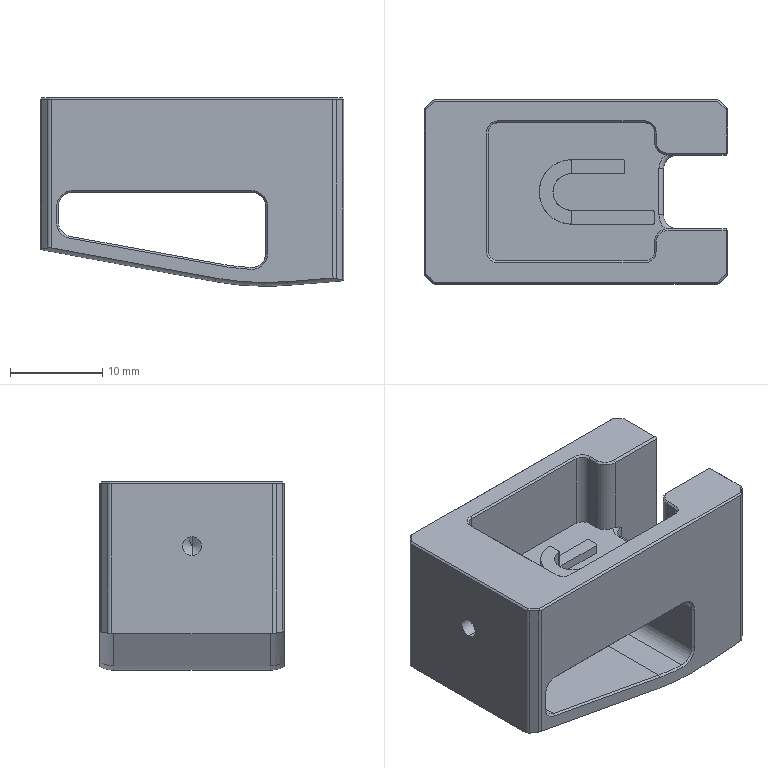NC program | NX | posted with a generic post | part box 33 x 20 x 20.478 mm
Lines 1298 to 2252 of 7616:
(FIXED_CONTOUR_COPY , TOOL : D2R0.5)
N2588 T24 M6
N2590 G54
N2592 G17 G0 G90 X-4.289 Y-10.746 B0. C0. S9500 M3
N2594 G43 Z30. H24
N2596 Z2.8
N2598 G94 G1 Z0.346 F1000.
N2600 X-4.343 Z0.091
N2602 X-4.461 Z-0.142
N2604 X-4.636 Z-0.336
N2606 X-4.854 Z-0.479
N2608 X-5.102 Z-0.56
N2610 X-5.363 Y-10.745 Z-0.574
N2612 X-5.715 Z-0.547 F2500.
N2614 X-6.315 Z-0.509
N2616 X-6.915 Y-10.744 Z-0.483
N2618 X-7.515 Z-0.47
N2620 X-8.115 Z-0.466
N2622 X-8.715 Y-10.743 Z-0.477
N2624 X-9.315 Z-0.496
N2626 X-9.915 Y-10.742 Z-0.532
N2628 X-10.515 Z-0.572
N2630 X-11.115 Z-0.62
N2632 X-11.715 Y-10.741 Z-0.668
N2634 X-12.315 Z-0.716
N2636 X-12.915 Y-10.74 Z-0.764
N2638 X-13.515 Z-0.812
N2640 X-14.115 Z-0.86
N2642 X-14.715 Y-10.739 Z-0.908
N2644 X-15.315 Z-0.956
N2646 X-15.495 Z-0.97
N2648 X-15.537 Y-10.719 Z-0.963
N2650 X-15.618 Y-10.705 Z-0.961
N2652 X-15.681 Y-10.646 Z-0.934
N2654 X-15.315 Z-0.905
N2656 X-14.715 Y-10.647 Z-0.857
N2658 X-14.115 Z-0.809
N2660 X-13.515 Z-0.762
N2662 X-12.915 Y-10.648 Z-0.714
N2664 X-12.315 Z-0.666
N2666 X-11.715 Y-10.649 Z-0.618
N2668 X-11.115 Z-0.57
N2670 X-10.515 Z-0.522
N2672 X-9.915 Y-10.65 Z-0.482
N2674 X-9.315 Z-0.446
N2676 X-8.715 Y-10.651 Z-0.428
N2678 X-8.115 Z-0.418
N2680 X-7.515 Z-0.42
N2682 X-6.915 Y-10.652 Z-0.435
N2684 X-6.315 Z-0.459
N2686 X-5.715 Y-10.653 Z-0.498
N2688 X-5.115 Z-0.547
N2690 X-4.515 Z-0.607
N2692 X-3.915 Y-10.654 Z-0.682
N2694 X-3.315 Z-0.765
N2696 X-2.715 Y-10.655 Z-0.865
N2698 X-2.115 Z-0.969
N2700 X-1.515 Z-1.08
N2702 X-0.915 Y-10.656 Z-1.19
N2704 X-0.315 Z-1.3
N2706 X0.285 Y-10.657 Z-1.411
N2708 X0.885 Z-1.521
N2710 X1.485 Z-1.631
N2712 X2.085 Y-10.658 Z-1.742
N2714 X2.685 Z-1.852
N2716 X3.285 Y-10.659 Z-1.962
N2718 X3.885 Z-2.073
N2720 X4.485 Z-2.183
N2722 X5.085 Y-10.66 Z-2.294
N2724 X5.685 Z-2.404
N2726 X6.285 Y-10.661 Z-2.514
N2728 X6.885 Z-2.625
N2730 X7.485 Z-2.735
N2732 X8.085 Y-10.662 Z-2.845
N2734 X8.685 Z-2.956
N2736 X9.285 Y-10.663 Z-3.066
N2738 X9.885 Z-3.176
N2740 X10.485 Z-3.287
N2742 X11.085 Y-10.664 Z-3.397
N2744 X11.685 Z-3.507
N2746 X12.285 Y-10.665 Z-3.617
N2748 X12.885 Z-3.728
N2750 X13.485 Z-3.838
N2752 X14.085 Y-10.666 Z-3.948
N2754 X14.685 Z-4.058
N2756 X15.285 Z-4.168
N2758 X15.762 Y-10.667 Z-4.256
N2760 X15.871 Y-10.567 Z-4.222
N2762 X15.286 Z-4.114
N2764 X14.686 Z-4.004
N2766 X14.086 Y-10.566 Z-3.894
N2768 X13.486 Z-3.783
N2770 X12.886 Y-10.565 Z-3.673
N2772 X12.286 Z-3.563
N2774 X11.686 Z-3.452
N2776 X11.086 Y-10.564 Z-3.342
N2778 X10.486 Z-3.232
N2780 X9.886 Y-10.563 Z-3.122
N2782 X9.286 Z-3.011
N2784 X8.686 Z-2.901
N2786 X8.086 Y-10.562 Z-2.791
N2788 X7.486 Z-2.68
N2790 X6.886 Y-10.561 Z-2.57
N2792 X6.286 Z-2.46
N2794 X5.686 Z-2.349
N2796 X5.086 Y-10.56 Z-2.239
N2798 X4.486 Z-2.129
N2800 X3.886 Y-10.559 Z-2.018
N2802 X3.286 Z-1.908
N2804 X2.686 Z-1.798
N2806 X2.086 Y-10.558 Z-1.687
N2808 X1.486 Z-1.577
N2810 X0.886 Y-10.557 Z-1.467
N2812 X0.286 Z-1.356
N2814 X-0.314 Z-1.246
N2816 X-0.914 Y-10.556 Z-1.136
N2818 X-1.514 Z-1.026
N2820 X-2.114 Y-10.555 Z-0.915
N2822 X-2.714 Z-0.811
N2824 X-3.314 Z-0.711
N2826 X-3.914 Y-10.554 Z-0.63
N2828 X-4.514 Z-0.555
N2830 X-5.114 Y-10.553 Z-0.495
N2832 X-5.714 Z-0.447
N2834 X-6.314 Z-0.406
N2836 X-6.914 Y-10.552 Z-0.384
N2838 X-7.514 Z-0.367
N2840 X-8.114 Y-10.551 Z-0.366
N2842 X-8.714 Z-0.375
N2844 X-9.314 Z-0.394
N2846 X-9.914 Y-10.55 Z-0.429
N2848 X-10.514 Z-0.468
N2850 X-11.114 Y-10.549 Z-0.517
N2852 X-11.714 Z-0.565
N2854 X-12.314 Z-0.613
N2856 X-12.914 Y-10.548 Z-0.661
N2858 X-13.514 Z-0.709
N2860 X-14.114 Y-10.547 Z-0.757
N2862 X-14.714 Z-0.805
N2864 X-15.314 Z-0.854
N2866 X-15.782 Y-10.546 Z-0.891
N2868 X-15.877 Y-10.447 Z-0.854
N2870 X-15.314 Z-0.809
N2872 X-14.714 Z-0.761
N2874 X-14.114 Y-10.448 Z-0.712
N2876 X-13.514 Z-0.664
N2878 X-12.914 Y-10.449 Z-0.615
N2880 X-12.314 Z-0.567
N2882 X-11.714 Z-0.519
N2884 X-11.114 Y-10.45 Z-0.471
N2886 X-10.514 Z-0.423
N2888 X-9.914 Y-10.451 Z-0.383
N2890 X-9.314 Z-0.348
N2892 X-8.714 Z-0.33
N2894 X-8.114 Y-10.452 Z-0.321
N2896 X-7.514 Z-0.322
N2898 X-6.914 Y-10.453 Z-0.338
N2900 X-6.314 Z-0.36
N2902 X-5.714 Z-0.401
N2904 X-5.114 Y-10.454 Z-0.449
N2906 X-4.514 Z-0.509
N2908 X-3.914 Y-10.455 Z-0.582
N2910 X-3.314 Z-0.663
N2912 X-2.714 Z-0.763
N2914 X-2.114 Y-10.456 Z-0.866
N2916 X-1.514 Z-0.977
N2918 X-0.914 Y-10.457 Z-1.087
N2920 X-0.314 Z-1.197
N2922 X0.286 Z-1.308
N2924 X0.886 Y-10.458 Z-1.418
N2926 X1.486 Z-1.528
N2928 X2.086 Y-10.459 Z-1.639
N2930 X2.686 Z-1.749
N2932 X3.286 Z-1.86
N2934 X3.886 Y-10.46 Z-1.97
N2936 X4.486 Z-2.08
N2938 X5.086 Y-10.461 Z-2.191
N2940 X5.686 Z-2.301
N2942 X6.286 Z-2.411
N2944 X6.886 Y-10.462 Z-2.522
N2946 X7.486 Z-2.632
N2948 X8.086 Y-10.463 Z-2.742
N2950 X8.686 Z-2.853
N2952 X9.286 Z-2.963
N2954 X9.886 Y-10.464 Z-3.073
N2956 X10.486 Z-3.184
N2958 X11.086 Y-10.465 Z-3.294
N2960 X11.686 Z-3.404
N2962 X12.286 Z-3.514
N2964 X12.886 Y-10.466 Z-3.625
N2966 X13.486 Z-3.735
N2968 X14.086 Y-10.467 Z-3.845
N2970 X14.686 Z-3.955
N2972 X15.286 Z-4.065
N2974 X15.886 Y-10.468 Z-4.176
N2976 X15.973 Z-4.192
N2978 X16.069 Y-10.368 Z-4.163
N2980 X15.886 Z-4.129
N2982 X15.286 Z-4.019
N2984 X14.686 Y-10.367 Z-3.908
N2986 X14.086 Z-3.798
N2988 X13.486 Z-3.688
N2990 X12.886 Y-10.366 Z-3.577
N2992 X12.286 Z-3.467
N2994 X11.686 Y-10.365 Z-3.357
N2996 X11.086 Z-3.246
N2998 X10.486 Z-3.136
N3000 X9.886 Y-10.364 Z-3.026
N3002 X9.286 Z-2.915
N3004 X8.686 Y-10.363 Z-2.805
N3006 X8.086 Z-2.695
N3008 X7.486 Z-2.585
N3010 X6.886 Y-10.362 Z-2.474
N3012 X6.286 Z-2.364
N3014 X5.686 Y-10.361 Z-2.254
N3016 X5.086 Z-2.144
N3018 X4.486 Z-2.033
N3020 X3.886 Y-10.36 Z-1.923
N3022 X3.286 Z-1.813
N3024 X2.686 Z-1.703
N3026 X2.086 Y-10.359 Z-1.593
N3028 X1.486 Z-1.482
N3030 X0.886 Y-10.358 Z-1.372
N3032 X0.286 Z-1.262
N3034 X-0.314 Z-1.151
N3036 X-0.914 Y-10.357 Z-1.041
N3038 X-1.514 Z-0.931
N3040 X-2.114 Y-10.356 Z-0.82
N3042 X-2.714 Z-0.717
N3044 X-3.314 Z-0.617
N3046 X-3.914 Y-10.355 Z-0.537
N3048 X-4.514 Z-0.463
N3050 X-5.114 Y-10.354 Z-0.403
N3052 X-5.714 Z-0.356
N3054 X-6.314 Z-0.315
N3056 X-6.914 Y-10.353 Z-0.293
N3058 X-7.514 Z-0.277
N3060 X-8.114 Y-10.352 Z-0.276
N3062 X-8.714 Z-0.285
N3064 X-9.314 Z-0.303
N3066 X-9.914 Y-10.351 Z-0.338
N3068 X-10.514 Z-0.377
N3070 X-11.114 Y-10.35 Z-0.426
N3072 X-11.714 Z-0.474
N3074 X-12.314 Z-0.522
N3076 X-12.914 Y-10.349 Z-0.571
N3078 X-13.514 Z-0.619
N3080 X-14.114 Y-10.348 Z-0.668
N3082 X-14.714 Z-0.716
N3084 X-15.314 Z-0.765
N3086 X-15.914 Y-10.347 Z-0.813
N3088 X-15.97 Z-0.818
N3090 X-16.063 Y-10.248 Z-0.781
N3092 X-15.914 Z-0.769
N3094 X-15.314 Z-0.722
N3096 X-14.714 Z-0.674
N3098 X-14.114 Y-10.249 Z-0.626
N3100 X-13.514 Z-0.578
N3102 X-12.914 Y-10.25 Z-0.53
N3104 X-12.314 Z-0.482
N3106 X-11.714 Z-0.434
N3108 X-11.114 Y-10.251 Z-0.386
N3110 X-10.514 Z-0.338
N3112 X-9.914 Y-10.252 Z-0.299
N3114 X-9.314 Z-0.265
N3116 X-8.714 Z-0.246
N3118 X-8.114 Y-10.253 Z-0.237
N3120 X-7.514 Z-0.238
N3122 X-6.914 Y-10.254 Z-0.254
N3124 X-6.314 Z-0.276
N3126 X-5.714 Z-0.316
N3128 X-5.114 Y-10.255 Z-0.363
N3130 X-4.514 Z-0.424
N3132 X-3.914 Y-10.256 Z-0.496
N3134 X-3.314 Z-0.576
N3136 X-2.714 Z-0.675
N3138 X-2.114 Y-10.257 Z-0.778
N3140 X-1.514 Z-0.888
N3142 X-0.914 Y-10.258 Z-0.999
N3144 X-0.314 Z-1.109
N3146 X0.286 Z-1.219
N3148 X0.886 Y-10.259 Z-1.33
N3150 X1.486 Z-1.44
N3152 X2.086 Y-10.26 Z-1.551
N3154 X2.686 Z-1.661
N3156 X3.286 Z-1.772
N3158 X3.886 Y-10.261 Z-1.882
N3160 X4.486 Z-1.992
N3162 X5.086 Y-10.262 Z-2.103
N3164 X5.686 Z-2.213
N3166 X6.286 Z-2.324
N3168 X6.886 Y-10.263 Z-2.434
N3170 X7.486 Z-2.545
N3172 X8.086 Y-10.264 Z-2.655
N3174 X8.686 Z-2.765
N3176 X9.286 Z-2.876
N3178 X9.886 Y-10.265 Z-2.986
N3180 X10.486 Z-3.097
N3182 X11.086 Y-10.266 Z-3.207
N3184 X11.686 Z-3.317
N3186 X12.286 Z-3.428
N3188 X12.886 Y-10.267 Z-3.538
N3190 X13.486 Z-3.648
N3192 X14.086 Y-10.268 Z-3.759
N3194 X14.686 Z-3.869
N3196 X15.286 Z-3.979
N3198 X15.886 Y-10.269 Z-4.09
N3200 X16.164 Z-4.141
N3202 X16.259 Y-10.169 Z-4.119
N3204 X15.886 Z-4.05
N3206 X15.286 Z-3.94
N3208 X14.686 Y-10.168 Z-3.83
N3210 X14.086 Z-3.719
N3212 X13.486 Z-3.609
N3214 X12.886 Y-10.167 Z-3.499
N3216 X12.286 Z-3.388
N3218 X11.686 Y-10.166 Z-3.278
N3220 X11.086 Z-3.168
N3222 X10.486 Z-3.057
N3224 X9.886 Y-10.165 Z-2.947
N3226 X9.286 Z-2.837
N3228 X8.686 Y-10.164 Z-2.726
N3230 X8.086 Z-2.616
N3232 X7.486 Z-2.506
N3234 X6.886 Y-10.163 Z-2.395
N3236 X6.286 Z-2.285
N3238 X5.686 Y-10.162 Z-2.175
N3240 X5.086 Z-2.064
N3242 X4.486 Z-1.954
N3244 X3.886 Y-10.161 Z-1.844
N3246 X3.286 Z-1.733
N3248 X2.686 Y-10.16 Z-1.623
N3250 X2.086 Z-1.513
N3252 X1.486 Z-1.402
N3254 X0.886 Y-10.159 Z-1.292
N3256 X0.286 Z-1.181
N3258 X-0.314 Y-10.158 Z-1.071
N3260 X-0.914 Z-0.961
N3262 X-1.514 Z-0.85
N3264 X-2.114 Y-10.157 Z-0.74
N3266 X-2.714 Z-0.637
N3268 X-3.314 Y-10.156 Z-0.538
N3270 X-3.914 Z-0.458
N3272 X-4.514 Z-0.386
N3274 X-5.114 Y-10.155 Z-0.326
N3276 X-5.714 Z-0.279
N3278 X-6.314 Y-10.154 Z-0.238
N3280 X-6.914 Z-0.217
N3282 X-7.514 Z-0.201
N3284 X-8.114 Y-10.153 Z-0.2
N3286 X-8.714 Z-0.209
N3288 X-9.314 Y-10.152 Z-0.227
N3290 X-9.914 Z-0.261
N3292 X-10.514 Z-0.3
N3294 X-11.114 Y-10.151 Z-0.348
N3296 X-11.714 Z-0.396
N3298 X-12.314 Y-10.15 Z-0.445
N3300 X-12.914 Z-0.493
N3302 X-13.514 Z-0.542
N3304 X-14.114 Y-10.149 Z-0.591
N3306 X-14.714 Z-0.64
N3308 X-15.314 Y-10.148 Z-0.688
N3310 X-15.914 Z-0.736
N3312 X-16.157 Z-0.755
N3314 X-16.251 Y-10.048 Z-0.73
N3316 X-15.914 Y-10.049 Z-0.703
N3318 X-15.314 Z-0.655
N3320 X-14.714 Z-0.607
N3322 X-14.114 Y-10.05 Z-0.559
N3324 X-13.514 Z-0.511
N3326 X-12.914 Y-10.051 Z-0.463
N3328 X-12.314 Z-0.414
N3330 X-11.714 Z-0.365
N3332 X-11.114 Y-10.052 Z-0.316
N3334 X-10.514 Z-0.267
N3336 X-9.914 Y-10.053 Z-0.228
N3338 X-9.314 Z-0.195
N3340 X-8.714 Z-0.176
N3342 X-8.114 Y-10.054 Z-0.168
N3344 X-7.514 Z-0.169
N3346 X-6.914 Y-10.055 Z-0.184
N3348 X-6.314 Z-0.206
N3350 X-5.714 Z-0.246
N3352 X-5.114 Y-10.056 Z-0.292
N3354 X-4.514 Z-0.352
N3356 X-3.914 Z-0.423
N3358 X-3.314 Y-10.057 Z-0.503
N3360 X-2.714 Z-0.6
N3362 X-2.114 Y-10.058 Z-0.702
N3364 X-1.514 Z-0.813
N3366 X-0.914 Z-0.923
N3368 X-0.314 Y-10.059 Z-1.033
N3370 X0.286 Z-1.144
N3372 X0.886 Y-10.06 Z-1.254
N3374 X1.486 Z-1.364
N3376 X2.086 Z-1.474
N3378 X2.686 Y-10.061 Z-1.585
N3380 X3.286 Z-1.695
N3382 X3.886 Y-10.062 Z-1.805
N3384 X4.486 Z-1.915
N3386 X5.086 Z-2.026
N3388 X5.686 Y-10.063 Z-2.136
N3390 X6.286 Z-2.246
N3392 X6.886 Y-10.064 Z-2.357
N3394 X7.486 Z-2.467
N3396 X8.086 Z-2.577
N3398 X8.686 Y-10.065 Z-2.687
N3400 X9.286 Z-2.798
N3402 X9.886 Y-10.066 Z-2.908
N3404 X10.486 Z-3.018
N3406 X11.086 Z-3.129
N3408 X11.686 Y-10.067 Z-3.239
N3410 X12.286 Z-3.349
N3412 X12.886 Y-10.068 Z-3.46
N3414 X13.486 Z-3.57
N3416 X14.086 Z-3.68
N3418 X14.686 Y-10.069 Z-3.791
N3420 X15.286 Z-3.901
N3422 X15.886 Y-10.07 Z-4.011
N3424 X16.354 Z-4.097
N3426 X16.448 Y-9.97 Z-4.082
N3428 X15.886 Z-3.979
N3430 X15.286 Z-3.868
N3432 X14.686 Y-9.969 Z-3.758
N3434 X14.086 Z-3.648
N3436 X13.486 Z-3.538
N3438 X12.886 Y-9.968 Z-3.427
N3440 X12.286 Z-3.317
N3442 X11.686 Y-9.967 Z-3.207
N3444 X11.086 Z-3.097
N3446 X10.486 Z-2.986
N3448 X9.886 Y-9.966 Z-2.876
N3450 X9.286 Z-2.766
N3452 X8.686 Y-9.965 Z-2.656
N3454 X8.086 Z-2.546
N3456 X7.486 Z-2.435
N3458 X6.886 Y-9.964 Z-2.325
N3460 X6.286 Z-2.215
N3462 X5.686 Y-9.963 Z-2.105
N3464 X5.086 Z-1.994
N3466 X4.486 Z-1.884
N3468 X3.886 Y-9.962 Z-1.774
N3470 X3.286 Z-1.664
N3472 X2.686 Y-9.961 Z-1.553
N3474 X2.086 Z-1.443
N3476 X1.486 Z-1.333
N3478 X0.886 Y-9.96 Z-1.223
N3480 X0.286 Z-1.112
N3482 X-0.314 Y-9.959 Z-1.002
N3484 X-0.914 Z-0.892
N3486 X-1.514 Z-0.782
N3488 X-2.114 Y-9.958 Z-0.672
N3490 X-2.714 Z-0.57
N3492 X-3.314 Y-9.957 Z-0.473
N3494 X-3.914 Z-0.393
N3496 X-4.514 Z-0.321
N3498 X-5.114 Y-9.956 Z-0.261
N3500 X-5.714 Z-0.215
N3502 X-6.314 Y-9.955 Z-0.175
N3504 X-6.914 Z-0.154
N3506 X-7.514 Z-0.138
N3508 X-8.114 Y-9.954 Z-0.137
N3510 X-8.714 Z-0.146
N3512 X-9.314 Y-9.953 Z-0.165
N3514 X-9.914 Z-0.198
N3516 X-10.514 Z-0.237
N3518 X-11.114 Y-9.952 Z-0.286
N3520 X-11.714 Z-0.334
N3522 X-12.314 Y-9.951 Z-0.382
N3524 X-12.914 Z-0.43
N3526 X-13.514 Z-0.478
N3528 X-14.114 Y-9.95 Z-0.526
N3530 X-14.714 Z-0.574
N3532 X-15.314 Y-9.949 Z-0.622
N3534 X-15.914 Z-0.67
N3536 X-16.345 Z-0.705
N3538 X-16.439 Y-9.849 Z-0.685
N3540 X-15.914 Z-0.643
N3542 X-15.314 Y-9.85 Z-0.595
N3544 X-14.714 Z-0.546
N3546 X-14.114 Y-9.851 Z-0.498
N3548 X-13.514 Z-0.45
N3550 X-12.914 Z-0.402
N3552 X-12.314 Y-9.852 Z-0.354
N3554 X-11.714 Z-0.305
N3556 X-11.114 Y-9.853 Z-0.257
N3558 X-10.514 Z-0.209
N3560 X-9.914 Z-0.171
N3562 X-9.314 Y-9.854 Z-0.138
N3564 X-8.714 Z-0.119
N3566 X-8.114 Y-9.855 Z-0.111
N3568 X-7.514 Z-0.112
N3570 X-6.914 Z-0.127
N3572 X-6.314 Y-9.856 Z-0.148
N3574 X-5.714 Z-0.188
N3576 X-5.114 Y-9.857 Z-0.232
N3578 X-4.514 Z-0.292
N3580 X-3.914 Z-0.363
N3582 X-3.314 Y-9.858 Z-0.443
N3584 X-2.714 Z-0.539
N3586 X-2.114 Y-9.859 Z-0.641
N3588 X-1.514 Z-0.751
N3590 X-0.914 Z-0.861
N3592 X-0.314 Y-9.86 Z-0.972
N3594 X0.286 Z-1.082
N3596 X0.886 Y-9.861 Z-1.192
N3598 X1.486 Z-1.302
N3600 X2.086 Z-1.413
N3602 X2.686 Y-9.862 Z-1.523
N3604 X3.286 Z-1.633
N3606 X3.886 Y-9.863 Z-1.743
N3608 X4.486 Z-1.854
N3610 X5.086 Z-1.964
N3612 X5.686 Y-9.864 Z-2.074
N3614 X6.286 Z-2.184
N3616 X6.886 Y-9.865 Z-2.295
N3618 X7.486 Z-2.405
N3620 X8.086 Z-2.515
N3622 X8.686 Y-9.866 Z-2.625
N3624 X9.286 Z-2.736
N3626 X9.886 Y-9.867 Z-2.846
N3628 X10.486 Z-2.956
N3630 X11.086 Z-3.066
N3632 X11.686 Y-9.868 Z-3.177
N3634 X12.286 Z-3.287
N3636 X12.886 Y-9.869 Z-3.397
N3638 X13.486 Z-3.508
N3640 X14.086 Z-3.618
N3642 X14.686 Y-9.87 Z-3.728
N3644 X15.286 Z-3.838
N3646 X15.886 Y-9.871 Z-3.949
N3648 X16.486 Z-4.059
N3650 X16.542 Z-4.069
N3652 X16.636 Y-9.772 Z-4.059
N3654 X16.486 Y-9.771 Z-4.031
N3656 X15.886 Z-3.921
N3658 X15.286 Z-3.811
N3660 X14.686 Y-9.77 Z-3.701
N3662 X14.086 Z-3.591
N3664 X13.486 Y-9.769 Z-3.48
N3666 X12.886 Z-3.37
N3668 X12.286 Z-3.26
N3670 X11.686 Y-9.768 Z-3.15
N3672 X11.086 Z-3.04
N3674 X10.486 Y-9.767 Z-2.929
N3676 X9.886 Z-2.819
N3678 X9.286 Z-2.709
N3680 X8.686 Y-9.766 Z-2.599
N3682 X8.086 Z-2.488
N3684 X7.486 Y-9.765 Z-2.378
N3686 X6.886 Z-2.268
N3688 X6.286 Z-2.158
N3690 X5.686 Y-9.764 Z-2.047
N3692 X5.086 Z-1.937
N3694 X4.486 Y-9.763 Z-1.827
N3696 X3.886 Z-1.717
N3698 X3.286 Z-1.607
N3700 X2.686 Y-9.762 Z-1.496
N3702 X2.086 Z-1.386
N3704 X1.486 Y-9.761 Z-1.276
N3706 X0.886 Z-1.166
N3708 X0.286 Z-1.055
N3710 X-0.314 Y-9.76 Z-0.945
N3712 X-0.914 Z-0.835
N3714 X-1.514 Y-9.759 Z-0.725
N3716 X-2.114 Z-0.615
N3718 X-2.714 Z-0.514
N3720 X-3.314 Y-9.758 Z-0.419
N3722 X-3.914 Z-0.339
N3724 X-4.514 Y-9.757 Z-0.269
N3726 X-5.114 Z-0.209
N3728 X-5.714 Z-0.164
N3730 X-6.314 Y-9.756 Z-0.125
N3732 X-6.914 Z-0.104
N3734 X-7.514 Y-9.755 Z-0.089
N3736 X-8.114 Z-0.088
N3738 X-8.714 Z-0.096
N3740 X-9.314 Y-9.754 Z-0.115
N3742 X-9.914 Z-0.147
N3744 X-10.514 Y-9.753 Z-0.186
N3746 X-11.114 Z-0.234
N3748 X-11.714 Z-0.282
N3750 X-12.314 Y-9.752 Z-0.33
N3752 X-12.914 Z-0.378
N3754 X-13.514 Y-9.751 Z-0.426
N3756 X-14.114 Z-0.474
N3758 X-14.714 Z-0.522
N3760 X-15.314 Y-9.75 Z-0.57
N3762 X-15.914 Z-0.618
N3764 X-16.514 Y-9.749 Z-0.666
N3766 X-16.53 Z-0.667
N3768 X-16.622 Y-9.65 Z-0.653
N3770 X-16.514 Z-0.644
N3772 X-15.914 Z-0.596
N3774 X-15.314 Y-9.651 Z-0.548
N3776 X-14.714 Z-0.5
N3778 X-14.114 Y-9.652 Z-0.452
N3780 X-13.514 Z-0.403
N3782 X-12.914 Z-0.355
N3784 X-12.314 Y-9.653 Z-0.307
N3786 X-11.714 Z-0.259
N3788 X-11.114 Y-9.654 Z-0.211
N3790 X-10.514 Z-0.163
N3792 X-9.914 Z-0.125
N3794 X-9.314 Y-9.655 Z-0.093
N3796 X-8.714 Z-0.074
N3798 X-8.114 Y-9.656 Z-0.066
N3800 X-7.514 Z-0.067
N3802 X-6.914 Z-0.082
N3804 X-6.314 Y-9.657 Z-0.103
N3806 X-5.714 Z-0.142
N3808 X-5.114 Y-9.658 Z-0.186
N3810 X-4.514 Z-0.246
N3812 X-3.914 Z-0.315
N3814 X-3.314 Y-9.659 Z-0.395
N3816 X-2.714 Z-0.49
N3818 X-2.114 Y-9.66 Z-0.591
N3820 X-1.514 Z-0.701
N3822 X-0.914 Z-0.811
N3824 X-0.314 Y-9.661 Z-0.922
N3826 X0.286 Z-1.032
N3828 X0.886 Y-9.662 Z-1.142
N3830 X1.486 Z-1.252
N3832 X2.086 Z-1.363
N3834 X2.686 Y-9.663 Z-1.473
N3836 X3.286 Z-1.583
N3838 X3.886 Y-9.664 Z-1.693
N3840 X4.486 Z-1.803
N3842 X5.086 Z-1.914
N3844 X5.686 Y-9.665 Z-2.024
N3846 X6.286 Z-2.134
N3848 X6.886 Z-2.244
N3850 X7.486 Y-9.666 Z-2.354
N3852 X8.086 Z-2.464
N3854 X8.686 Y-9.667 Z-2.575
N3856 X9.286 Z-2.685
N3858 X9.886 Z-2.795
N3860 X10.486 Y-9.668 Z-2.905
N3862 X11.086 Z-3.015
N3864 X11.686 Y-9.669 Z-3.125
N3866 X12.286 Z-3.236
N3868 X12.886 Z-3.346
N3870 X13.486 Y-9.67 Z-3.456
N3872 X14.086 Z-3.566
N3874 X14.686 Y-9.671 Z-3.676
N3876 X15.286 Z-3.786
N3878 X15.886 Z-3.897
N3880 X16.486 Y-9.672 Z-4.007
N3882 X16.721 Z-4.05
N3884 X16.79 Y-9.591 Z-4.044
N3886 X16.802 Y-9.573 Z-4.043
N3888 X16.486 Y-9.572 Z-3.985
N3890 X15.886 Z-3.875
N3892 X15.286 Z-3.764
N3894 X14.686 Y-9.571 Z-3.654
N3896 X14.086 Z-3.544
N3898 X13.486 Y-9.57 Z-3.434
N3900 X12.886 Z-3.323
N3902 X12.286 Z-3.213
N3904 X11.686 Y-9.569 Z-3.103
N3906 X11.086 Z-2.993
N3908 X10.486 Y-9.568 Z-2.883
N3910 X9.886 Z-2.772
N3912 X9.286 Z-2.662
N3914 X8.686 Y-9.567 Z-2.552
N3916 X8.086 Z-2.442
N3918 X7.486 Y-9.566 Z-2.331
N3920 X6.886 Z-2.221
N3922 X6.286 Z-2.111
N3924 X5.686 Y-9.565 Z-2.001
N3926 X5.086 Z-1.891
N3928 X4.486 Y-9.564 Z-1.78
N3930 X3.886 Z-1.67
N3932 X3.286 Z-1.56
N3934 X2.686 Y-9.563 Z-1.45
N3936 X2.086 Z-1.339
N3938 X1.486 Y-9.562 Z-1.229
N3940 X0.886 Z-1.119
N3942 X0.286 Z-1.009
N3944 X-0.314 Y-9.561 Z-0.899
N3946 X-0.914 Z-0.788
N3948 X-1.514 Y-9.56 Z-0.678
N3950 X-2.114 Z-0.568
N3952 X-2.714 Z-0.468
N3954 X-3.314 Y-9.559 Z-0.374
N3956 X-3.914 Z-0.294
N3958 X-4.514 Y-9.558 Z-0.227
N3960 X-5.114 Z-0.167
N3962 X-5.714 Z-0.125
N3964 X-6.314 Y-9.557 Z-0.086
N3966 X-6.914 Z-0.066
N3968 X-7.514 Y-9.556 Z-0.051
N3970 X-8.114 Z-0.05
N3972 X-8.714 Z-0.058
N3974 X-9.314 Y-9.555 Z-0.077
N3976 X-9.914 Z-0.108
N3978 X-10.514 Y-9.554 Z-0.146
N3980 X-11.114 Z-0.193
N3982 X-11.714 Z-0.242
N3984 X-12.314 Y-9.553 Z-0.29
N3986 X-12.914 Z-0.338
N3988 X-13.514 Y-9.552 Z-0.386
N3990 X-14.114 Z-0.434
N3992 X-14.714 Z-0.482
N3994 X-15.314 Y-9.551 Z-0.53
N3996 X-15.914 Z-0.578
N3998 X-16.514 Y-9.55 Z-0.626
N4000 X-16.704 Z-0.641
N4002 X-16.74 Y-9.506 Z-0.637
N4004 X-16.763 Y-9.451 Z-0.63
N4006 X-16.514 Z-0.61
N4008 X-15.914 Z-0.562
N4010 X-15.314 Y-9.452 Z-0.514
N4012 X-14.714 Z-0.465
N4014 X-14.114 Z-0.417
N4016 X-13.514 Y-9.453 Z-0.369
N4018 X-12.914 Z-0.321
N4020 X-12.314 Y-9.454 Z-0.273
N4022 X-11.714 Z-0.225
N4024 X-11.114 Z-0.177
N4026 X-10.514 Y-9.455 Z-0.13
N4028 X-9.914 Z-0.091
N4030 X-9.314 Y-9.456 Z-0.06
N4032 X-8.714 Z-0.041
N4034 X-8.114 Z-0.034
N4036 X-7.514 Y-9.457 Z-0.035
N4038 X-6.914 Z-0.049
N4040 X-6.314 Y-9.458 Z-0.07
N4042 X-5.714 Z-0.108
N4044 X-5.114 Z-0.151
N4046 X-4.514 Y-9.459 Z-0.211
N4048 X-3.914 Z-0.278
N4050 X-3.314 Y-9.46 Z-0.358
N4052 X-2.714 Z-0.45
N4054 X-2.114 Z-0.551
N4056 X-1.514 Y-9.461 Z-0.66
N4058 X-0.914 Z-0.77
N4060 X-0.314 Y-9.462 Z-0.881
N4062 X0.286 Z-0.991
N4064 X0.886 Z-1.101
N4066 X1.486 Y-9.463 Z-1.211
N4068 X2.086 Z-1.321
N4070 X2.686 Y-9.464 Z-1.432
N4072 X3.286 Z-1.542
N4074 X3.886 Z-1.652
N4076 X4.486 Y-9.465 Z-1.762
N4078 X5.086 Z-1.872
N4080 X5.686 Y-9.466 Z-1.983
N4082 X6.286 Z-2.093
N4084 X6.886 Z-2.203
N4086 X7.486 Y-9.467 Z-2.313
N4088 X8.086 Z-2.423
N4090 X8.686 Y-9.468 Z-2.533
N4092 X9.286 Z-2.644
N4094 X9.886 Z-2.754
N4096 X10.486 Y-9.469 Z-2.864
N4098 X11.086 Z-2.974
N4100 X11.686 Y-9.47 Z-3.084
N4102 X12.286 Z-3.195
N4104 X12.886 Z-3.305
N4106 X13.486 Y-9.471 Z-3.415
N4108 X14.086 Z-3.525
N4110 X14.686 Y-9.472 Z-3.635
N4112 X15.286 Z-3.745
N4114 X15.886 Z-3.855
N4116 X16.486 Y-9.473 Z-3.966
N4118 X16.866 Z-4.035
N4120 X16.93 Y-9.374 Z-4.03
N4122 X16.486 Y-9.373 Z-3.948
N4124 X15.886 Z-3.838
N4126 X15.286 Y-9.372 Z-3.728
N4128 X14.686 Z-3.618
N4130 X14.086 Z-3.508
N4132 X13.486 Y-9.371 Z-3.397
N4134 X12.886 Z-3.287
N4136 X12.286 Y-9.37 Z-3.177
N4138 X11.686 Z-3.067
N4140 X11.086 Z-2.957
N4142 X10.486 Y-9.369 Z-2.847
N4144 X9.886 Z-2.736
N4146 X9.286 Y-9.368 Z-2.626
N4148 X8.686 Z-2.516
N4150 X8.086 Z-2.406
N4152 X7.486 Y-9.367 Z-2.296
N4154 X6.886 Z-2.186
N4156 X6.286 Y-9.366 Z-2.076
N4158 X5.686 Z-1.965
N4160 X5.086 Z-1.855
N4162 X4.486 Y-9.365 Z-1.745
N4164 X3.886 Z-1.635
N4166 X3.286 Y-9.364 Z-1.525
N4168 X2.686 Z-1.415
N4170 X2.086 Z-1.305
N4172 X1.486 Y-9.363 Z-1.195
N4174 X0.886 Z-1.084
N4176 X0.286 Y-9.362 Z-0.974
N4178 X-0.314 Z-0.864
N4180 X-0.914 Z-0.754
N4182 X-1.514 Y-9.361 Z-0.644
N4184 X-2.114 Z-0.534
N4186 X-2.714 Y-9.36 Z-0.434
N4188 X-3.314 Z-0.341
N4190 X-3.914 Z-0.261
N4192 X-4.514 Y-9.359 Z-0.195
N4194 X-5.114 Z-0.135
N4196 X-5.714 Y-9.358 Z-0.094
N4198 X-6.314 Z-0.059
N4200 X-6.914 Z-0.038
N4202 X-7.514 Y-9.357 Z-0.023
N4204 X-8.114 Z-0.022
N4206 X-8.714 Z-0.031
N4208 X-9.314 Y-9.356 Z-0.049
N4210 X-9.914 Z-0.078
N4212 X-10.514 Y-9.355 Z-0.117
N4214 X-11.114 Z-0.162
N4216 X-11.714 Z-0.211
N4218 X-12.314 Y-9.354 Z-0.259
N4220 X-12.914 Z-0.307
N4222 X-13.514 Y-9.353 Z-0.355
N4224 X-14.114 Z-0.403
N4226 X-14.714 Z-0.452
N4228 X-15.314 Y-9.352 Z-0.5
N4230 X-15.914 Z-0.548
N4232 X-16.514 Y-9.351 Z-0.596
N4234 X-16.804 Z-0.62
N4236 X-16.843 Y-9.252 Z-0.611
N4238 X-16.514 Z-0.585
N4240 X-15.914 Z-0.537
N4242 X-15.314 Y-9.253 Z-0.489
N4244 X-14.714 Z-0.441
N4246 X-14.114 Z-0.393
N4248 X-13.514 Y-9.254 Z-0.345
N4250 X-12.914 Z-0.297
N4252 X-12.314 Y-9.255 Z-0.249
N4254 X-11.714 Z-0.201
N4256 X-11.114 Z-0.152
N4258 X-10.514 Y-9.256 Z-0.107
N4260 X-9.914 Z-0.068
N4262 X-9.314 Y-9.257 Z-0.04
N4264 X-8.714 Z-0.021
N4266 X-8.114 Z-0.011
N4268 X-7.514 Y-9.258 Z-0.014
N4270 X-6.914 Z-0.028
N4272 X-6.314 Y-9.259 Z-0.049
N4274 X-5.714 Z-0.085
N4276 X-5.114 Z-0.125
N4278 X-4.514 Y-9.26 Z-0.184
N4280 X-3.914 Z-0.248
N4282 X-3.314 Y-9.261 Z-0.328
N4284 X-2.714 Z-0.419
N4286 X-2.114 Z-0.519
N4288 X-1.514 Y-9.262 Z-0.628
N4290 X-0.914 Z-0.738
N4292 X-0.314 Y-9.263 Z-0.848
N4294 X0.286 Z-0.958
N4296 X0.886 Z-1.068
N4298 X1.486 Y-9.264 Z-1.179
N4300 X2.086 Z-1.289
N4302 X2.686 Y-9.265 Z-1.399
N4304 X3.286 Z-1.509
N4306 X3.886 Z-1.619
N4308 X4.486 Y-9.266 Z-1.73
N4310 X5.086 Z-1.84
N4312 X5.686 Y-9.267 Z-1.95
N4314 X6.286 Z-2.06
N4316 X6.886 Z-2.17
N4318 X7.486 Y-9.268 Z-2.28
N4320 X8.086 Z-2.391
N4322 X8.686 Y-9.269 Z-2.501
N4324 X9.286 Z-2.611
N4326 X9.886 Z-2.721
N4328 X10.486 Y-9.27 Z-2.831
N4330 X11.086 Z-2.942
N4332 X11.686 Y-9.271 Z-3.052
N4334 X12.286 Z-3.162
N4336 X12.886 Z-3.272
N4338 X13.486 Y-9.272 Z-3.382
N4340 X14.086 Z-3.493
N4342 X14.686 Z-3.603
N4344 X15.286 Y-9.273 Z-3.713
N4346 X15.886 Z-3.823
N4348 X16.486 Y-9.274 Z-3.933
N4350 X16.966 Z-4.021
N4352 X16.991 Y-9.174 Z-4.014
N4354 X16.486 Z-3.921
N4356 X15.886 Z-3.811
N4358 X15.286 Y-9.173 Z-3.701
N4360 X14.686 Z-3.59
N4362 X14.086 Z-3.48
N4364 X13.486 Y-9.172 Z-3.37
N4366 X12.886 Z-3.26
N4368 X12.286 Y-9.171 Z-3.15
N4370 X11.686 Z-3.04
N4372 X11.086 Z-2.929
N4374 X10.486 Y-9.17 Z-2.819
N4376 X9.886 Z-2.709
N4378 X9.286 Y-9.169 Z-2.599
N4380 X8.686 Z-2.489
N4382 X8.086 Z-2.378
N4384 X7.486 Y-9.168 Z-2.268
N4386 X6.886 Z-2.158
N4388 X6.286 Y-9.167 Z-2.048
N4390 X5.686 Z-1.938
N4392 X5.086 Z-1.828
N4394 X4.486 Y-9.166 Z-1.717
N4396 X3.886 Z-1.607
N4398 X3.286 Y-9.165 Z-1.497
N4400 X2.686 Z-1.387
N4402 X2.086 Z-1.277
N4404 X1.486 Y-9.164 Z-1.167
N4406 X0.886 Z-1.057
N4408 X0.286 Y-9.163 Z-0.946
N4410 X-0.314 Z-0.836
N4412 X-0.914 Z-0.726
N4414 X-1.514 Y-9.162 Z-0.616
N4416 X-2.114 Z-0.508
N4418 X-2.714 Y-9.161 Z-0.408
N4420 X-3.314 Z-0.318
N4422 X-3.914 Z-0.238
N4424 X-4.514 Y-9.16 Z-0.174
N4426 X-5.114 Z-0.115
N4428 X-5.714 Y-9.159 Z-0.075
N4430 X-6.314 Z-0.041
N4432 X-6.914 Z-0.02
N4434 X-7.514 Y-9.158 Z-0.008
N4436 X-8.114 Z-0.006
N4438 X-8.714 Y-9.157 Z-0.013
N4440 X-9.314 Z-0.031
N4442 X-9.914 Z-0.059
N4444 X-10.514 Y-9.156 Z-0.097
N4446 X-11.114 Z-0.142
N4448 X-11.714 Y-9.155 Z-0.191
N4450 X-12.314 Z-0.239
N4452 X-12.914 Z-0.287
N4454 X-13.514 Y-9.154 Z-0.335
N4456 X-14.114 Z-0.383
N4458 X-14.714 Y-9.153 Z-0.431
N4460 X-15.314 Z-0.479
N4462 X-15.914 Z-0.528
N4464 X-16.514 Y-9.152 Z-0.576
N4466 X-16.882 Z-0.606
N4468 X-16.921 Y-9.052 Z-0.602
N4470 X-16.513 Y-9.053 Z-0.569
N4472 X-15.913 Z-0.52
N4474 X-15.313 Z-0.472
N4476 X-14.713 Y-9.054 Z-0.424
N4478 X-14.113 Z-0.375
N4480 X-13.513 Y-9.055 Z-0.327
N4482 X-12.913 Z-0.279
N4484 X-12.313 Z-0.231
N4486 X-11.713 Y-9.056 Z-0.182
N4488 X-11.113 Z-0.134
N4490 X-10.513 Y-9.057 Z-0.09